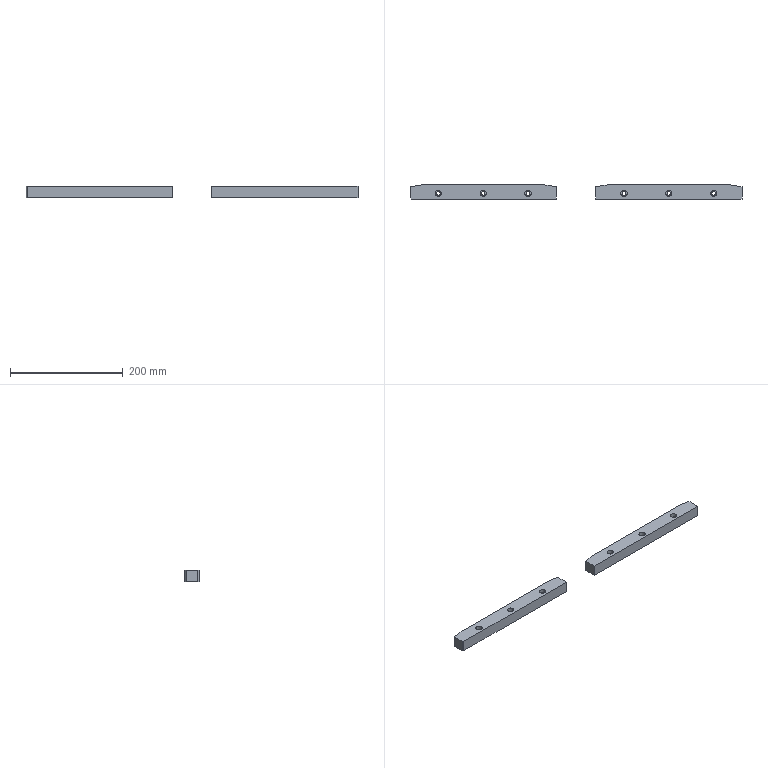Part | SolidWorks | features BaseBody 2 | 2 solids | 47 faces | box 588 x 25 x 20 mm | volume 249973 mm3 | cylinder 24 | plane 23 | commonest cylinder face diameters 6.6 x12 11 x12
STEP:
#1=CARTESIAN_POINT('',(180.,-11.723,13.2));
#2=VERTEX_POINT('',#1);
#3=CARTESIAN_POINT('',(191.,-11.723,13.2));
#4=VERTEX_POINT('',#3);
#5=CARTESIAN_POINT('',(185.5,-11.723,13.2));
#6=DIRECTION('',(0.,0.,1.));
#7=DIRECTION('',(1.,0.,0.));
#8=AXIS2_PLACEMENT_3D('',#5,#6,#7);
#9=CIRCLE('',#8,5.5);
#10=EDGE_CURVE('',#2,#4,#9,.T.);
#11=ORIENTED_EDGE('',*,*,#10,.F.);
#12=CARTESIAN_POINT('',(180.,-11.723,20.));
#13=VERTEX_POINT('',#12);
#14=CARTESIAN_POINT('',(180.,-11.723,20.));
#15=DIRECTION('',(0.,0.,1.));
#16=VECTOR('',#15,1000.);
#17=LINE('',#14,#16);
#18=EDGE_CURVE('',#2,#13,#17,.T.);
#19=ORIENTED_EDGE('',*,*,#18,.T.);
#20=CARTESIAN_POINT('',(191.,-11.723,20.));
#21=VERTEX_POINT('',#20);
#22=CARTESIAN_POINT('',(185.5,-11.723,20.));
#23=DIRECTION('',(0.,0.,1.));
#24=DIRECTION('',(1.,0.,0.));
#25=AXIS2_PLACEMENT_3D('',#22,#23,#24);
#26=CIRCLE('',#25,5.5);
#27=EDGE_CURVE('',#13,#21,#26,.T.);
#28=ORIENTED_EDGE('',*,*,#27,.T.);
#29=CARTESIAN_POINT('',(191.,-11.723,20.));
#30=DIRECTION('',(0.,0.,1.));
#31=VECTOR('',#30,1000.);
#32=LINE('',#29,#31);
#33=EDGE_CURVE('',#4,#21,#32,.T.);
#34=ORIENTED_EDGE('',*,*,#33,.F.);
#35=EDGE_LOOP('',(#11,#19,#28,#34));
#36=FACE_OUTER_BOUND('',#35,.T.);
#37=CARTESIAN_POINT('',(185.5,-11.723,20.));
#38=DIRECTION('',(0.,0.,1.));
#39=DIRECTION('',(1.,0.,0.));
#40=AXIS2_PLACEMENT_3D('',#37,#38,#39);
#41=CYLINDRICAL_SURFACE('',#40,5.5);
#42=ADVANCED_FACE('',(#36),#41,.F.);
#43=CARTESIAN_POINT('',(182.2,-11.723,0.));
#44=VERTEX_POINT('',#43);
#45=CARTESIAN_POINT('',(188.8,-11.723,0.));
#46=VERTEX_POINT('',#45);
#47=CARTESIAN_POINT('',(185.5,-11.723,0.));
#48=DIRECTION('',(0.,0.,1.));
#49=DIRECTION('',(1.,0.,0.));
#50=AXIS2_PLACEMENT_3D('',#47,#48,#49);
#51=CIRCLE('',#50,3.3);
#52=EDGE_CURVE('',#44,#46,#51,.T.);
#53=ORIENTED_EDGE('',*,*,#52,.F.);
#54=CARTESIAN_POINT('',(182.2,-11.723,13.2));
#55=VERTEX_POINT('',#54);
#56=CARTESIAN_POINT('',(182.2,-11.723,20.));
#57=DIRECTION('',(0.,0.,1.));
#58=VECTOR('',#57,1000.);
#59=LINE('',#56,#58);
#60=EDGE_CURVE('',#44,#55,#59,.T.);
#61=ORIENTED_EDGE('',*,*,#60,.T.);
#62=CARTESIAN_POINT('',(188.8,-11.723,13.2));
#63=VERTEX_POINT('',#62);
#64=CARTESIAN_POINT('',(185.5,-11.723,13.2));
#65=DIRECTION('',(0.,0.,1.));
#66=DIRECTION('',(1.,0.,0.));
#67=AXIS2_PLACEMENT_3D('',#64,#65,#66);
#68=CIRCLE('',#67,3.3);
#69=EDGE_CURVE('',#55,#63,#68,.T.);
#70=ORIENTED_EDGE('',*,*,#69,.T.);
#71=CARTESIAN_POINT('',(188.8,-11.723,20.));
#72=DIRECTION('',(0.,0.,1.));
#73=VECTOR('',#72,1000.);
#74=LINE('',#71,#73);
#75=EDGE_CURVE('',#46,#63,#74,.T.);
#76=ORIENTED_EDGE('',*,*,#75,.F.);
#77=EDGE_LOOP('',(#53,#61,#70,#76));
#78=FACE_OUTER_BOUND('',#77,.T.);
#79=CARTESIAN_POINT('',(185.5,-11.723,20.));
#80=DIRECTION('',(0.,0.,1.));
#81=DIRECTION('',(1.,0.,0.));
#82=AXIS2_PLACEMENT_3D('',#79,#80,#81);
#83=CYLINDRICAL_SURFACE('',#82,3.3);
#84=ADVANCED_FACE('',(#78),#83,.F.);
#85=CARTESIAN_POINT('',(259.5,-11.723,13.2));
#86=VERTEX_POINT('',#85);
#87=CARTESIAN_POINT('',(270.5,-11.723,13.2));
#88=VERTEX_POINT('',#87);
#89=CARTESIAN_POINT('',(265.,-11.723,13.2));
#90=DIRECTION('',(0.,0.,1.));
#91=DIRECTION('',(1.,0.,0.));
#92=AXIS2_PLACEMENT_3D('',#89,#90,#91);
#93=CIRCLE('',#92,5.5);
#94=EDGE_CURVE('',#86,#88,#93,.T.);
#95=ORIENTED_EDGE('',*,*,#94,.F.);
#96=CARTESIAN_POINT('',(259.5,-11.723,20.));
#97=VERTEX_POINT('',#96);
#98=CARTESIAN_POINT('',(259.5,-11.723,20.));
#99=DIRECTION('',(0.,0.,1.));
#100=VECTOR('',#99,1000.);
#101=LINE('',#98,#100);
#102=EDGE_CURVE('',#86,#97,#101,.T.);
#103=ORIENTED_EDGE('',*,*,#102,.T.);
#104=CARTESIAN_POINT('',(270.5,-11.723,20.));
#105=VERTEX_POINT('',#104);
#106=CARTESIAN_POINT('',(265.,-11.723,20.));
#107=DIRECTION('',(0.,0.,1.));
#108=DIRECTION('',(1.,0.,0.));
#109=AXIS2_PLACEMENT_3D('',#106,#107,#108);
#110=CIRCLE('',#109,5.5);
#111=EDGE_CURVE('',#97,#105,#110,.T.);
#112=ORIENTED_EDGE('',*,*,#111,.T.);
#113=CARTESIAN_POINT('',(270.5,-11.723,20.));
#114=DIRECTION('',(0.,0.,1.));
#115=VECTOR('',#114,1000.);
#116=LINE('',#113,#115);
#117=EDGE_CURVE('',#88,#105,#116,.T.);
#118=ORIENTED_EDGE('',*,*,#117,.F.);
#119=EDGE_LOOP('',(#95,#103,#112,#118));
#120=FACE_OUTER_BOUND('',#119,.T.);
#121=CARTESIAN_POINT('',(265.,-11.723,20.));
#122=DIRECTION('',(0.,0.,1.));
#123=DIRECTION('',(1.,0.,0.));
#124=AXIS2_PLACEMENT_3D('',#121,#122,#123);
#125=CYLINDRICAL_SURFACE('',#124,5.5);
#126=ADVANCED_FACE('',(#120),#125,.F.);
#127=CARTESIAN_POINT('',(261.7,-11.723,0.));
#128=VERTEX_POINT('',#127);
#129=CARTESIAN_POINT('',(268.3,-11.723,0.));
#130=VERTEX_POINT('',#129);
#131=CARTESIAN_POINT('',(265.,-11.723,0.));
#132=DIRECTION('',(0.,0.,1.));
#133=DIRECTION('',(1.,0.,0.));
#134=AXIS2_PLACEMENT_3D('',#131,#132,#133);
#135=CIRCLE('',#134,3.3);
#136=EDGE_CURVE('',#128,#130,#135,.T.);
#137=ORIENTED_EDGE('',*,*,#136,.F.);
#138=CARTESIAN_POINT('',(261.7,-11.723,13.2));
#139=VERTEX_POINT('',#138);
#140=CARTESIAN_POINT('',(261.7,-11.723,20.));
#141=DIRECTION('',(0.,0.,1.));
#142=VECTOR('',#141,1000.);
#143=LINE('',#140,#142);
#144=EDGE_CURVE('',#128,#139,#143,.T.);
#145=ORIENTED_EDGE('',*,*,#144,.T.);
#146=CARTESIAN_POINT('',(268.3,-11.723,13.2));
#147=VERTEX_POINT('',#146);
#148=CARTESIAN_POINT('',(265.,-11.723,13.2));
#149=DIRECTION('',(0.,0.,1.));
#150=DIRECTION('',(1.,0.,0.));
#151=AXIS2_PLACEMENT_3D('',#148,#149,#150);
#152=CIRCLE('',#151,3.3);
#153=EDGE_CURVE('',#139,#147,#152,.T.);
#154=ORIENTED_EDGE('',*,*,#153,.T.);
#155=CARTESIAN_POINT('',(268.3,-11.723,20.));
#156=DIRECTION('',(0.,0.,1.));
#157=VECTOR('',#156,1000.);
#158=LINE('',#155,#157);
#159=EDGE_CURVE('',#130,#147,#158,.T.);
#160=ORIENTED_EDGE('',*,*,#159,.F.);
#161=EDGE_LOOP('',(#137,#145,#154,#160));
#162=FACE_OUTER_BOUND('',#161,.T.);
#163=CARTESIAN_POINT('',(265.,-11.723,20.));
#164=DIRECTION('',(0.,0.,1.));
#165=DIRECTION('',(1.,0.,0.));
#166=AXIS2_PLACEMENT_3D('',#163,#164,#165);
#167=CYLINDRICAL_SURFACE('',#166,3.3);
#168=ADVANCED_FACE('',(#162),#167,.F.);
#169=CARTESIAN_POINT('',(100.5,-11.723,13.2));
#170=VERTEX_POINT('',#169);
#171=CARTESIAN_POINT('',(111.5,-11.723,13.2));
#172=VERTEX_POINT('',#171);
#173=CARTESIAN_POINT('',(106.,-11.723,13.2));
#174=DIRECTION('',(0.,0.,1.));
#175=DIRECTION('',(1.,0.,0.));
#176=AXIS2_PLACEMENT_3D('',#173,#174,#175);
#177=CIRCLE('',#176,5.5);
#178=EDGE_CURVE('',#170,#172,#177,.T.);
#179=ORIENTED_EDGE('',*,*,#178,.F.);
#180=CARTESIAN_POINT('',(100.5,-11.723,20.));
#181=VERTEX_POINT('',#180);
#182=CARTESIAN_POINT('',(100.5,-11.723,20.));
#183=DIRECTION('',(0.,0.,1.));
#184=VECTOR('',#183,1000.);
#185=LINE('',#182,#184);
#186=EDGE_CURVE('',#170,#181,#185,.T.);
#187=ORIENTED_EDGE('',*,*,#186,.T.);
#188=CARTESIAN_POINT('',(111.5,-11.723,20.));
#189=VERTEX_POINT('',#188);
#190=CARTESIAN_POINT('',(106.,-11.723,20.));
#191=DIRECTION('',(0.,0.,1.));
#192=DIRECTION('',(1.,0.,0.));
#193=AXIS2_PLACEMENT_3D('',#190,#191,#192);
#194=CIRCLE('',#193,5.5);
#195=EDGE_CURVE('',#181,#189,#194,.T.);
#196=ORIENTED_EDGE('',*,*,#195,.T.);
#197=CARTESIAN_POINT('',(111.5,-11.723,20.));
#198=DIRECTION('',(0.,0.,1.));
#199=VECTOR('',#198,1000.);
#200=LINE('',#197,#199);
#201=EDGE_CURVE('',#172,#189,#200,.T.);
#202=ORIENTED_EDGE('',*,*,#201,.F.);
#203=EDGE_LOOP('',(#179,#187,#196,#202));
#204=FACE_OUTER_BOUND('',#203,.T.);
#205=CARTESIAN_POINT('',(106.,-11.723,20.));
#206=DIRECTION('',(0.,0.,1.));
#207=DIRECTION('',(1.,0.,0.));
#208=AXIS2_PLACEMENT_3D('',#205,#206,#207);
#209=CYLINDRICAL_SURFACE('',#208,5.5);
#210=ADVANCED_FACE('',(#204),#209,.F.);
#211=CARTESIAN_POINT('',(102.7,-11.723,0.));
#212=VERTEX_POINT('',#211);
#213=CARTESIAN_POINT('',(109.3,-11.723,0.));
#214=VERTEX_POINT('',#213);
#215=CARTESIAN_POINT('',(106.,-11.723,0.));
#216=DIRECTION('',(0.,0.,1.));
#217=DIRECTION('',(1.,0.,0.));
#218=AXIS2_PLACEMENT_3D('',#215,#216,#217);
#219=CIRCLE('',#218,3.3);
#220=EDGE_CURVE('',#212,#214,#219,.T.);
#221=ORIENTED_EDGE('',*,*,#220,.F.);
#222=CARTESIAN_POINT('',(102.7,-11.723,13.2));
#223=VERTEX_POINT('',#222);
#224=CARTESIAN_POINT('',(102.7,-11.723,20.));
#225=DIRECTION('',(0.,0.,1.));
#226=VECTOR('',#225,1000.);
#227=LINE('',#224,#226);
#228=EDGE_CURVE('',#212,#223,#227,.T.);
#229=ORIENTED_EDGE('',*,*,#228,.T.);
#230=CARTESIAN_POINT('',(109.3,-11.723,13.2));
#231=VERTEX_POINT('',#230);
#232=CARTESIAN_POINT('',(106.,-11.723,13.2));
#233=DIRECTION('',(0.,0.,1.));
#234=DIRECTION('',(1.,0.,0.));
#235=AXIS2_PLACEMENT_3D('',#232,#233,#234);
#236=CIRCLE('',#235,3.3);
#237=EDGE_CURVE('',#223,#231,#236,.T.);
#238=ORIENTED_EDGE('',*,*,#237,.T.);
#239=CARTESIAN_POINT('',(109.3,-11.723,20.));
#240=DIRECTION('',(0.,0.,1.));
#241=VECTOR('',#240,1000.);
#242=LINE('',#239,#241);
#243=EDGE_CURVE('',#214,#231,#242,.T.);
#244=ORIENTED_EDGE('',*,*,#243,.F.);
#245=EDGE_LOOP('',(#221,#229,#238,#244));
#246=FACE_OUTER_BOUND('',#245,.T.);
#247=CARTESIAN_POINT('',(106.,-11.723,20.));
#248=DIRECTION('',(0.,0.,1.));
#249=DIRECTION('',(1.,0.,0.));
#250=AXIS2_PLACEMENT_3D('',#247,#248,#249);
#251=CYLINDRICAL_SURFACE('',#250,3.3);
#252=ADVANCED_FACE('',(#246),#251,.F.);
#253=CARTESIAN_POINT('',(295.,3.277,0.));
#254=VERTEX_POINT('',#253);
#255=CARTESIAN_POINT('',(76.,3.277,0.));
#256=VERTEX_POINT('',#255);
#257=CARTESIAN_POINT('',(-253.,3.277,0.));
#258=DIRECTION('',(-1.,0.,0.));
#259=VECTOR('',#258,1000.);
#260=LINE('',#257,#259);
#261=EDGE_CURVE('',#254,#256,#260,.T.);
#262=ORIENTED_EDGE('',*,*,#261,.T.);
#263=CARTESIAN_POINT('',(76.,3.277,20.));
#264=VERTEX_POINT('',#263);
#265=CARTESIAN_POINT('',(76.,3.277,20.));
#266=DIRECTION('',(0.,0.,1.));
#267=VECTOR('',#266,1000.);
#268=LINE('',#265,#267);
#269=EDGE_CURVE('',#256,#264,#268,.T.);
#270=ORIENTED_EDGE('',*,*,#269,.T.);
#271=CARTESIAN_POINT('',(295.,3.277,20.));
#272=VERTEX_POINT('',#271);
#273=CARTESIAN_POINT('',(-253.,3.277,20.));
#274=DIRECTION('',(-1.,0.,0.));
#275=VECTOR('',#274,1000.);
#276=LINE('',#273,#275);
#277=EDGE_CURVE('',#272,#264,#276,.T.);
#278=ORIENTED_EDGE('',*,*,#277,.F.);
#279=CARTESIAN_POINT('',(295.,3.277,20.));
#280=DIRECTION('',(0.,0.,-1.));
#281=VECTOR('',#280,1000.);
#282=LINE('',#279,#281);
#283=EDGE_CURVE('',#272,#254,#282,.T.);
#284=ORIENTED_EDGE('',*,*,#283,.T.);
#285=EDGE_LOOP('',(#262,#270,#278,#284));
#286=FACE_OUTER_BOUND('',#285,.T.);
#287=CARTESIAN_POINT('',(-253.,3.277,20.));
#288=DIRECTION('',(0.,-1.,0.));
#289=DIRECTION('',(1.,0.,0.));
#290=AXIS2_PLACEMENT_3D('',#287,#288,#289);
#291=PLANE('',#290);
#292=ADVANCED_FACE('',(#286),#291,.F.);
#293=CARTESIAN_POINT('',(56.,-21.723,20.));
#294=VERTEX_POINT('',#293);
#295=CARTESIAN_POINT('',(315.,-21.723,20.));
#296=VERTEX_POINT('',#295);
#297=CARTESIAN_POINT('',(-271.,-21.723,20.));
#298=DIRECTION('',(1.,0.,0.));
#299=VECTOR('',#298,1000.);
#300=LINE('',#297,#299);
#301=EDGE_CURVE('',#294,#296,#300,.T.);
#302=ORIENTED_EDGE('',*,*,#301,.F.);
#303=CARTESIAN_POINT('',(56.,-21.723,0.));
#304=VERTEX_POINT('',#303);
#305=CARTESIAN_POINT('',(56.,-21.723,20.));
#306=DIRECTION('',(0.,0.,-1.));
#307=VECTOR('',#306,1000.);
#308=LINE('',#305,#307);
#309=EDGE_CURVE('',#294,#304,#308,.T.);
#310=ORIENTED_EDGE('',*,*,#309,.T.);
#311=CARTESIAN_POINT('',(315.,-21.723,0.));
#312=VERTEX_POINT('',#311);
#313=CARTESIAN_POINT('',(-271.,-21.723,0.));
#314=DIRECTION('',(1.,0.,0.));
#315=VECTOR('',#314,1000.);
#316=LINE('',#313,#315);
#317=EDGE_CURVE('',#304,#312,#316,.T.);
#318=ORIENTED_EDGE('',*,*,#317,.T.);
#319=CARTESIAN_POINT('',(315.,-21.723,20.));
#320=DIRECTION('',(0.,0.,-1.));
#321=VECTOR('',#320,1000.);
#322=LINE('',#319,#321);
#323=EDGE_CURVE('',#296,#312,#322,.T.);
#324=ORIENTED_EDGE('',*,*,#323,.F.);
#325=EDGE_LOOP('',(#302,#310,#318,#324));
#326=FACE_OUTER_BOUND('',#325,.T.);
#327=CARTESIAN_POINT('',(-271.,-21.723,20.));
#328=DIRECTION('',(0.,1.,0.));
#329=DIRECTION('',(-1.,0.,0.));
#330=AXIS2_PLACEMENT_3D('',#327,#328,#329);
#331=PLANE('',#330);
#332=ADVANCED_FACE('',(#326),#331,.F.);
#333=CARTESIAN_POINT('',(106.,-11.723,20.));
#334=DIRECTION('',(0.,0.,1.));
#335=DIRECTION('',(1.,0.,0.));
#336=AXIS2_PLACEMENT_3D('',#333,#334,#335);
#337=CIRCLE('',#336,5.5);
#338=EDGE_CURVE('',#189,#181,#337,.T.);
#339=ORIENTED_EDGE('',*,*,#338,.F.);
#340=ORIENTED_EDGE('',*,*,#195,.F.);
#341=EDGE_LOOP('',(#339,#340));
#342=FACE_BOUND('',#341,.T.);
#343=CARTESIAN_POINT('',(265.,-11.723,20.));
#344=DIRECTION('',(0.,0.,1.));
#345=DIRECTION('',(1.,0.,0.));
#346=AXIS2_PLACEMENT_3D('',#343,#344,#345);
#347=CIRCLE('',#346,5.5);
#348=EDGE_CURVE('',#105,#97,#347,.T.);
#349=ORIENTED_EDGE('',*,*,#348,.F.);
#350=ORIENTED_EDGE('',*,*,#111,.F.);
#351=EDGE_LOOP('',(#349,#350));
#352=FACE_BOUND('',#351,.T.);
#353=CARTESIAN_POINT('',(185.5,-11.723,20.));
#354=DIRECTION('',(0.,0.,1.));
#355=DIRECTION('',(1.,0.,0.));
#356=AXIS2_PLACEMENT_3D('',#353,#354,#355);
#357=CIRCLE('',#356,5.5);
#358=EDGE_CURVE('',#21,#13,#357,.T.);
#359=ORIENTED_EDGE('',*,*,#358,.F.);
#360=ORIENTED_EDGE('',*,*,#27,.F.);
#361=EDGE_LOOP('',(#359,#360));
#362=FACE_BOUND('',#361,.T.);
#363=ORIENTED_EDGE('',*,*,#277,.T.);
#364=CARTESIAN_POINT('',(56.,0.2766,20.));
#365=VERTEX_POINT('',#364);
#366=CARTESIAN_POINT('',(76.,3.277,20.));
#367=DIRECTION('',(-0.9889,-0.1483,0.));
#368=VECTOR('',#367,1000.);
#369=LINE('',#366,#368);
#370=EDGE_CURVE('',#264,#365,#369,.T.);
#371=ORIENTED_EDGE('',*,*,#370,.T.);
#372=CARTESIAN_POINT('',(56.,-54.685,20.));
#373=DIRECTION('',(0.,1.,0.));
#374=VECTOR('',#373,1000.);
#375=LINE('',#372,#374);
#376=EDGE_CURVE('',#294,#365,#375,.T.);
#377=ORIENTED_EDGE('',*,*,#376,.F.);
#378=ORIENTED_EDGE('',*,*,#301,.T.);
#379=CARTESIAN_POINT('',(315.,0.2766,20.));
#380=VERTEX_POINT('',#379);
#381=CARTESIAN_POINT('',(315.,0.2766,20.));
#382=DIRECTION('',(0.,1.,0.));
#383=VECTOR('',#382,1000.);
#384=LINE('',#381,#383);
#385=EDGE_CURVE('',#296,#380,#384,.T.);
#386=ORIENTED_EDGE('',*,*,#385,.T.);
#387=CARTESIAN_POINT('',(295.,3.277,20.));
#388=DIRECTION('',(-0.9889,0.1483,0.));
#389=VECTOR('',#388,1000.);
#390=LINE('',#387,#389);
#391=EDGE_CURVE('',#380,#272,#390,.T.);
#392=ORIENTED_EDGE('',*,*,#391,.T.);
#393=EDGE_LOOP('',(#363,#371,#377,#378,#386,#392));
#394=FACE_OUTER_BOUND('',#393,.T.);
#395=CARTESIAN_POINT('',(0.,0.,20.));
#396=DIRECTION('',(0.,0.,-1.));
#397=DIRECTION('',(-1.,0.,0.));
#398=AXIS2_PLACEMENT_3D('',#395,#396,#397);
#399=PLANE('',#398);
#400=ADVANCED_FACE('',(#342,#352,#362,#394),#399,.F.);
#401=CARTESIAN_POINT('',(56.,0.2766,0.));
#402=VERTEX_POINT('',#401);
#403=CARTESIAN_POINT('',(56.,0.,0.));
#404=DIRECTION('',(0.,-1.,0.));
#405=VECTOR('',#404,1000.);
#406=LINE('',#403,#405);
#407=EDGE_CURVE('',#402,#304,#406,.T.);
#408=ORIENTED_EDGE('',*,*,#407,.F.);
#409=CARTESIAN_POINT('',(1.192,-7.945,0.));
#410=DIRECTION('',(0.9889,0.1483,0.));
#411=VECTOR('',#410,1000.);
#412=LINE('',#409,#411);
#413=EDGE_CURVE('',#402,#256,#412,.T.);
#414=ORIENTED_EDGE('',*,*,#413,.T.);
#415=ORIENTED_EDGE('',*,*,#261,.F.);
#416=CARTESIAN_POINT('',(315.,0.2766,0.));
#417=VERTEX_POINT('',#416);
#418=CARTESIAN_POINT('',(295.,3.277,0.));
#419=DIRECTION('',(-0.9889,0.1483,0.));
#420=VECTOR('',#419,1000.);
#421=LINE('',#418,#420);
#422=EDGE_CURVE('',#417,#254,#421,.T.);
#423=ORIENTED_EDGE('',*,*,#422,.F.);
#424=CARTESIAN_POINT('',(315.,0.2766,0.));
#425=DIRECTION('',(0.,1.,0.));
#426=VECTOR('',#425,1000.);
#427=LINE('',#424,#426);
#428=EDGE_CURVE('',#312,#417,#427,.T.);
#429=ORIENTED_EDGE('',*,*,#428,.F.);
#430=ORIENTED_EDGE('',*,*,#317,.F.);
#431=EDGE_LOOP('',(#408,#414,#415,#423,#429,#430));
#432=FACE_OUTER_BOUND('',#431,.T.);
#433=CARTESIAN_POINT('',(106.,-11.723,0.));
#434=DIRECTION('',(0.,0.,1.));
#435=DIRECTION('',(1.,0.,0.));
#436=AXIS2_PLACEMENT_3D('',#433,#434,#435);
#437=CIRCLE('',#436,3.3);
#438=EDGE_CURVE('',#214,#212,#437,.T.);
#439=ORIENTED_EDGE('',*,*,#438,.T.);
#440=ORIENTED_EDGE('',*,*,#220,.T.);
#441=EDGE_LOOP('',(#439,#440));
#442=FACE_BOUND('',#441,.T.);
#443=CARTESIAN_POINT('',(265.,-11.723,0.));
#444=DIRECTION('',(0.,0.,1.));
#445=DIRECTION('',(1.,0.,0.));
#446=AXIS2_PLACEMENT_3D('',#443,#444,#445);
#447=CIRCLE('',#446,3.3);
#448=EDGE_CURVE('',#130,#128,#447,.T.);
#449=ORIENTED_EDGE('',*,*,#448,.T.);
#450=ORIENTED_EDGE('',*,*,#136,.T.);
#451=EDGE_LOOP('',(#449,#450));
#452=FACE_BOUND('',#451,.T.);
#453=CARTESIAN_POINT('',(185.5,-11.723,0.));
#454=DIRECTION('',(0.,0.,1.));
#455=DIRECTION('',(1.,0.,0.));
#456=AXIS2_PLACEMENT_3D('',#453,#454,#455);
#457=CIRCLE('',#456,3.3);
#458=EDGE_CURVE('',#46,#44,#457,.T.);
#459=ORIENTED_EDGE('',*,*,#458,.T.);
#460=ORIENTED_EDGE('',*,*,#52,.T.);
#461=EDGE_LOOP('',(#459,#460));
#462=FACE_BOUND('',#461,.T.);
#463=CARTESIAN_POINT('',(0.,0.,0.));
#464=DIRECTION('',(0.,0.,-1.));
#465=DIRECTION('',(-1.,0.,0.));
#466=AXIS2_PLACEMENT_3D('',#463,#464,#465);
#467=PLANE('',#466);
#468=ADVANCED_FACE('',(#432,#442,#452,#462),#467,.T.);
#469=ORIENTED_EDGE('',*,*,#422,.T.);
#470=ORIENTED_EDGE('',*,*,#283,.F.);
#471=ORIENTED_EDGE('',*,*,#391,.F.);
#472=CARTESIAN_POINT('',(315.,0.2766,20.));
#473=DIRECTION('',(0.,0.,-1.));
#474=VECTOR('',#473,1000.);
#475=LINE('',#472,#474);
#476=EDGE_CURVE('',#380,#417,#475,.T.);
#477=ORIENTED_EDGE('',*,*,#476,.T.);
#478=EDGE_LOOP('',(#469,#470,#471,#477));
#479=FACE_OUTER_BOUND('',#478,.T.);
#480=CARTESIAN_POINT('',(295.,3.277,20.));
#481=DIRECTION('',(-0.1483,-0.9889,0.));
#482=DIRECTION('',(0.9889,-0.1483,0.));
#483=AXIS2_PLACEMENT_3D('',#480,#481,#482);
#484=PLANE('',#483);
#485=ADVANCED_FACE('',(#479),#484,.F.);
#486=ORIENTED_EDGE('',*,*,#428,.T.);
#487=ORIENTED_EDGE('',*,*,#476,.F.);
#488=ORIENTED_EDGE('',*,*,#385,.F.);
#489=ORIENTED_EDGE('',*,*,#323,.T.);
#490=EDGE_LOOP('',(#486,#487,#488,#489));
#491=FACE_OUTER_BOUND('',#490,.T.);
#492=CARTESIAN_POINT('',(315.,0.2766,20.));
#493=DIRECTION('',(-1.,0.,0.));
#494=DIRECTION('',(0.,-1.,0.));
#495=AXIS2_PLACEMENT_3D('',#492,#493,#494);
#496=PLANE('',#495);
#497=ADVANCED_FACE('',(#491),#496,.F.);
#498=ORIENTED_EDGE('',*,*,#228,.F.);
#499=ORIENTED_EDGE('',*,*,#438,.F.);
#500=ORIENTED_EDGE('',*,*,#243,.T.);
#501=CARTESIAN_POINT('',(106.,-11.723,13.2));
#502=DIRECTION('',(0.,0.,1.));
#503=DIRECTION('',(1.,0.,0.));
#504=AXIS2_PLACEMENT_3D('',#501,#502,#503);
#505=CIRCLE('',#504,3.3);
#506=EDGE_CURVE('',#231,#223,#505,.T.);
#507=ORIENTED_EDGE('',*,*,#506,.T.);
#508=EDGE_LOOP('',(#498,#499,#500,#507));
#509=FACE_OUTER_BOUND('',#508,.T.);
#510=CARTESIAN_POINT('',(106.,-11.723,20.));
#511=DIRECTION('',(0.,0.,1.));
#512=DIRECTION('',(1.,0.,0.));
#513=AXIS2_PLACEMENT_3D('',#510,#511,#512);
#514=CYLINDRICAL_SURFACE('',#513,3.3);
#515=ADVANCED_FACE('',(#509),#514,.F.);
#516=ORIENTED_EDGE('',*,*,#506,.F.);
#517=ORIENTED_EDGE('',*,*,#237,.F.);
#518=EDGE_LOOP('',(#516,#517));
#519=FACE_BOUND('',#518,.T.);
#520=CARTESIAN_POINT('',(106.,-11.723,13.2));
#521=DIRECTION('',(0.,0.,1.));
#522=DIRECTION('',(1.,0.,0.));
#523=AXIS2_PLACEMENT_3D('',#520,#521,#522);
#524=CIRCLE('',#523,5.5);
#525=EDGE_CURVE('',#172,#170,#524,.T.);
#526=ORIENTED_EDGE('',*,*,#525,.T.);
#527=ORIENTED_EDGE('',*,*,#178,.T.);
#528=EDGE_LOOP('',(#526,#527));
#529=FACE_OUTER_BOUND('',#528,.T.);
#530=CARTESIAN_POINT('',(109.3,-11.723,13.2));
#531=DIRECTION('',(0.,0.,-1.));
#532=DIRECTION('',(-1.,0.,0.));
#533=AXIS2_PLACEMENT_3D('',#530,#531,#532);
#534=PLANE('',#533);
#535=ADVANCED_FACE('',(#519,#529),#534,.F.);
#536=ORIENTED_EDGE('',*,*,#186,.F.);
#537=ORIENTED_EDGE('',*,*,#525,.F.);
#538=ORIENTED_EDGE('',*,*,#201,.T.);
#539=ORIENTED_EDGE('',*,*,#338,.T.);
#540=EDGE_LOOP('',(#536,#537,#538,#539));
#541=FACE_OUTER_BOUND('',#540,.T.);
#542=CARTESIAN_POINT('',(106.,-11.723,20.));
#543=DIRECTION('',(0.,0.,1.));
#544=DIRECTION('',(1.,0.,0.));
#545=AXIS2_PLACEMENT_3D('',#542,#543,#544);
#546=CYLINDRICAL_SURFACE('',#545,5.5);
#547=ADVANCED_FACE('',(#541),#546,.F.);
#548=ORIENTED_EDGE('',*,*,#144,.F.);
#549=ORIENTED_EDGE('',*,*,#448,.F.);
#550=ORIENTED_EDGE('',*,*,#159,.T.);
#551=CARTESIAN_POINT('',(265.,-11.723,13.2));
#552=DIRECTION('',(0.,0.,1.));
#553=DIRECTION('',(1.,0.,0.));
#554=AXIS2_PLACEMENT_3D('',#551,#552,#553);
#555=CIRCLE('',#554,3.3);
#556=EDGE_CURVE('',#147,#139,#555,.T.);
#557=ORIENTED_EDGE('',*,*,#556,.T.);
#558=EDGE_LOOP('',(#548,#549,#550,#557));
#559=FACE_OUTER_BOUND('',#558,.T.);
#560=CARTESIAN_POINT('',(265.,-11.723,20.));
#561=DIRECTION('',(0.,0.,1.));
#562=DIRECTION('',(1.,0.,0.));
#563=AXIS2_PLACEMENT_3D('',#560,#561,#562);
#564=CYLINDRICAL_SURFACE('',#563,3.3);
#565=ADVANCED_FACE('',(#559),#564,.F.);
#566=ORIENTED_EDGE('',*,*,#556,.F.);
#567=ORIENTED_EDGE('',*,*,#153,.F.);
#568=EDGE_LOOP('',(#566,#567));
#569=FACE_BOUND('',#568,.T.);
#570=CARTESIAN_POINT('',(265.,-11.723,13.2));
#571=DIRECTION('',(0.,0.,1.));
#572=DIRECTION('',(1.,0.,0.));
#573=AXIS2_PLACEMENT_3D('',#570,#571,#572);
#574=CIRCLE('',#573,5.5);
#575=EDGE_CURVE('',#88,#86,#574,.T.);
#576=ORIENTED_EDGE('',*,*,#575,.T.);
#577=ORIENTED_EDGE('',*,*,#94,.T.);
#578=EDGE_LOOP('',(#576,#577));
#579=FACE_OUTER_BOUND('',#578,.T.);
#580=CARTESIAN_POINT('',(268.3,-11.723,13.2));
#581=DIRECTION('',(0.,0.,-1.));
#582=DIRECTION('',(-1.,0.,0.));
#583=AXIS2_PLACEMENT_3D('',#580,#581,#582);
#584=PLANE('',#583);
#585=ADVANCED_FACE('',(#569,#579),#584,.F.);
#586=ORIENTED_EDGE('',*,*,#102,.F.);
#587=ORIENTED_EDGE('',*,*,#575,.F.);
#588=ORIENTED_EDGE('',*,*,#117,.T.);
#589=ORIENTED_EDGE('',*,*,#348,.T.);
#590=EDGE_LOOP('',(#586,#587,#588,#589));
#591=FACE_OUTER_BOUND('',#590,.T.);
#592=CARTESIAN_POINT('',(265.,-11.723,20.));
#593=DIRECTION('',(0.,0.,1.));
#594=DIRECTION('',(1.,0.,0.));
#595=AXIS2_PLACEMENT_3D('',#592,#593,#594);
#596=CYLINDRICAL_SURFACE('',#595,5.5);
#597=ADVANCED_FACE('',(#591),#596,.F.);
#598=ORIENTED_EDGE('',*,*,#60,.F.);
#599=ORIENTED_EDGE('',*,*,#458,.F.);
#600=ORIENTED_EDGE('',*,*,#75,.T.);
#601=CARTESIAN_POINT('',(185.5,-11.723,13.2));
#602=DIRECTION('',(0.,0.,1.));
#603=DIRECTION('',(1.,0.,0.));
#604=AXIS2_PLACEMENT_3D('',#601,#602,#603);
#605=CIRCLE('',#604,3.3);
#606=EDGE_CURVE('',#63,#55,#605,.T.);
#607=ORIENTED_EDGE('',*,*,#606,.T.);
#608=EDGE_LOOP('',(#598,#599,#600,#607));
#609=FACE_OUTER_BOUND('',#608,.T.);
#610=CARTESIAN_POINT('',(185.5,-11.723,20.));
#611=DIRECTION('',(0.,0.,1.));
#612=DIRECTION('',(1.,0.,0.));
#613=AXIS2_PLACEMENT_3D('',#610,#611,#612);
#614=CYLINDRICAL_SURFACE('',#613,3.3);
#615=ADVANCED_FACE('',(#609),#614,.F.);
#616=ORIENTED_EDGE('',*,*,#606,.F.);
#617=ORIENTED_EDGE('',*,*,#69,.F.);
#618=EDGE_LOOP('',(#616,#617));
#619=FACE_BOUND('',#618,.T.);
#620=CARTESIAN_POINT('',(185.5,-11.723,13.2));
#621=DIRECTION('',(0.,0.,1.));
#622=DIRECTION('',(1.,0.,0.));
#623=AXIS2_PLACEMENT_3D('',#620,#621,#622);
#624=CIRCLE('',#623,5.5);
#625=EDGE_CURVE('',#4,#2,#624,.T.);
#626=ORIENTED_EDGE('',*,*,#625,.T.);
#627=ORIENTED_EDGE('',*,*,#10,.T.);
#628=EDGE_LOOP('',(#626,#627));
#629=FACE_OUTER_BOUND('',#628,.T.);
#630=CARTESIAN_POINT('',(188.8,-11.723,13.2));
#631=DIRECTION('',(0.,0.,-1.));
#632=DIRECTION('',(-1.,0.,0.));
#633=AXIS2_PLACEMENT_3D('',#630,#631,#632);
#634=PLANE('',#633);
#635=ADVANCED_FACE('',(#619,#629),#634,.F.);
#636=ORIENTED_EDGE('',*,*,#18,.F.);
#637=ORIENTED_EDGE('',*,*,#625,.F.);
#638=ORIENTED_EDGE('',*,*,#33,.T.);
#639=ORIENTED_EDGE('',*,*,#358,.T.);
#640=EDGE_LOOP('',(#636,#637,#638,#639));
#641=FACE_OUTER_BOUND('',#640,.T.);
#642=CARTESIAN_POINT('',(185.5,-11.723,20.));
#643=DIRECTION('',(0.,0.,1.));
#644=DIRECTION('',(1.,0.,0.));
#645=AXIS2_PLACEMENT_3D('',#642,#643,#644);
#646=CYLINDRICAL_SURFACE('',#645,5.5);
#647=ADVANCED_FACE('',(#641),#646,.F.);
#648=ORIENTED_EDGE('',*,*,#376,.T.);
#649=CARTESIAN_POINT('',(56.,0.2766,0.));
#650=DIRECTION('',(0.,0.,-1.));
#651=VECTOR('',#650,1000.);
#652=LINE('',#649,#651);
#653=EDGE_CURVE('',#365,#402,#652,.T.);
#654=ORIENTED_EDGE('',*,*,#653,.T.);
#655=ORIENTED_EDGE('',*,*,#407,.T.);
#656=ORIENTED_EDGE('',*,*,#309,.F.);
#657=EDGE_LOOP('',(#648,#654,#655,#656));
#658=FACE_OUTER_BOUND('',#657,.T.);
#659=CARTESIAN_POINT('',(56.,-54.685,0.));
#660=DIRECTION('',(1.,0.,0.));
#661=DIRECTION('',(0.,0.,-1.));
#662=AXIS2_PLACEMENT_3D('',#659,#660,#661);
#663=PLANE('',#662);
#664=ADVANCED_FACE('',(#658),#663,.F.);
#665=ORIENTED_EDGE('',*,*,#413,.F.);
#666=ORIENTED_EDGE('',*,*,#653,.F.);
#667=ORIENTED_EDGE('',*,*,#370,.F.);
#668=ORIENTED_EDGE('',*,*,#269,.F.);
#669=EDGE_LOOP('',(#665,#666,#667,#668));
#670=FACE_OUTER_BOUND('',#669,.T.);
#671=CARTESIAN_POINT('',(76.,3.277,20.));
#672=DIRECTION('',(0.1483,-0.9889,0.));
#673=DIRECTION('',(0.,0.,1.));
#674=AXIS2_PLACEMENT_3D('',#671,#672,#673);
#675=PLANE('',#674);
#676=ADVANCED_FACE('',(#670),#675,.F.);
#677=CLOSED_SHELL('',(#42,#84,#126,#168,#210,#252,#292,#332,#400,#468,#485,#497,#515,#535,#547,#565,#585,#597,#615,#635,#647,#664,#676));
#678=MANIFOLD_SOLID_BREP('',#677);
#679=CARTESIAN_POINT('',(-226.3,-11.723,0.));
#680=VERTEX_POINT('',#679);
#681=CARTESIAN_POINT('',(-219.7,-11.723,0.));
#682=VERTEX_POINT('',#681);
#683=CARTESIAN_POINT('',(-223.,-11.723,0.));
#684=DIRECTION('',(0.,0.,1.));
#685=DIRECTION('',(1.,0.,0.));
#686=AXIS2_PLACEMENT_3D('',#683,#684,#685);
#687=CIRCLE('',#686,3.3);
#688=EDGE_CURVE('',#680,#682,#687,.T.);
#689=ORIENTED_EDGE('',*,*,#688,.F.);
#690=CARTESIAN_POINT('',(-226.3,-11.723,13.2));
#691=VERTEX_POINT('',#690);
#692=CARTESIAN_POINT('',(-226.3,-11.723,20.));
#693=DIRECTION('',(0.,0.,1.));
#694=VECTOR('',#693,1000.);
#695=LINE('',#692,#694);
#696=EDGE_CURVE('',#680,#691,#695,.T.);
#697=ORIENTED_EDGE('',*,*,#696,.T.);
#698=CARTESIAN_POINT('',(-219.7,-11.723,13.2));
#699=VERTEX_POINT('',#698);
#700=CARTESIAN_POINT('',(-223.,-11.723,13.2));
#701=DIRECTION('',(0.,0.,1.));
#702=DIRECTION('',(1.,0.,0.));
#703=AXIS2_PLACEMENT_3D('',#700,#701,#702);
#704=CIRCLE('',#703,3.3);
#705=EDGE_CURVE('',#691,#699,#704,.T.);
#706=ORIENTED_EDGE('',*,*,#705,.T.);
#707=CARTESIAN_POINT('',(-219.7,-11.723,20.));
#708=DIRECTION('',(0.,0.,1.));
#709=VECTOR('',#708,1000.);
#710=LINE('',#707,#709);
#711=EDGE_CURVE('',#682,#699,#710,.T.);
#712=ORIENTED_EDGE('',*,*,#711,.F.);
#713=EDGE_LOOP('',(#689,#697,#706,#712));
#714=FACE_OUTER_BOUND('',#713,.T.);
#715=CARTESIAN_POINT('',(-223.,-11.723,20.));
#716=DIRECTION('',(0.,0.,1.));
#717=DIRECTION('',(1.,0.,0.));
#718=AXIS2_PLACEMENT_3D('',#715,#716,#717);
#719=CYLINDRICAL_SURFACE('',#718,3.3);
#720=ADVANCED_FACE('',(#714),#719,.F.);
#721=CARTESIAN_POINT('',(-146.8,-11.723,0.));
#722=VERTEX_POINT('',#721);
#723=CARTESIAN_POINT('',(-140.2,-11.723,0.));
#724=VERTEX_POINT('',#723);
#725=CARTESIAN_POINT('',(-143.5,-11.723,0.));
#726=DIRECTION('',(0.,0.,1.));
#727=DIRECTION('',(1.,0.,0.));
#728=AXIS2_PLACEMENT_3D('',#725,#726,#727);
#729=CIRCLE('',#728,3.3);
#730=EDGE_CURVE('',#722,#724,#729,.T.);
#731=ORIENTED_EDGE('',*,*,#730,.F.);
#732=CARTESIAN_POINT('',(-146.8,-11.723,13.2));
#733=VERTEX_POINT('',#732);
#734=CARTESIAN_POINT('',(-146.8,-11.723,20.));
#735=DIRECTION('',(0.,0.,1.));
#736=VECTOR('',#735,1000.);
#737=LINE('',#734,#736);
#738=EDGE_CURVE('',#722,#733,#737,.T.);
#739=ORIENTED_EDGE('',*,*,#738,.T.);
#740=CARTESIAN_POINT('',(-140.2,-11.723,13.2));
#741=VERTEX_POINT('',#740);
#742=CARTESIAN_POINT('',(-143.5,-11.723,13.2));
#743=DIRECTION('',(0.,0.,1.));
#744=DIRECTION('',(1.,0.,0.));
#745=AXIS2_PLACEMENT_3D('',#742,#743,#744);
#746=CIRCLE('',#745,3.3);
#747=EDGE_CURVE('',#733,#741,#746,.T.);
#748=ORIENTED_EDGE('',*,*,#747,.T.);
#749=CARTESIAN_POINT('',(-140.2,-11.723,20.));
#750=DIRECTION('',(0.,0.,1.));
#751=VECTOR('',#750,1000.);
#752=LINE('',#749,#751);
#753=EDGE_CURVE('',#724,#741,#752,.T.);
#754=ORIENTED_EDGE('',*,*,#753,.F.);
#755=EDGE_LOOP('',(#731,#739,#748,#754));
#756=FACE_OUTER_BOUND('',#755,.T.);
#757=CARTESIAN_POINT('',(-143.5,-11.723,20.));
#758=DIRECTION('',(0.,0.,1.));
#759=DIRECTION('',(1.,0.,0.));
#760=AXIS2_PLACEMENT_3D('',#757,#758,#759);
#761=CYLINDRICAL_SURFACE('',#760,3.3);
#762=ADVANCED_FACE('',(#756),#761,.F.);
#763=CARTESIAN_POINT('',(-67.3,-11.723,0.));
#764=VERTEX_POINT('',#763);
#765=CARTESIAN_POINT('',(-60.7,-11.723,0.));
#766=VERTEX_POINT('',#765);
#767=CARTESIAN_POINT('',(-64.,-11.723,0.));
#768=DIRECTION('',(0.,0.,1.));
#769=DIRECTION('',(1.,0.,0.));
#770=AXIS2_PLACEMENT_3D('',#767,#768,#769);
#771=CIRCLE('',#770,3.3);
#772=EDGE_CURVE('',#764,#766,#771,.T.);
#773=ORIENTED_EDGE('',*,*,#772,.F.);
#774=CARTESIAN_POINT('',(-67.3,-11.723,13.2));
#775=VERTEX_POINT('',#774);
#776=CARTESIAN_POINT('',(-67.3,-11.723,20.));
#777=DIRECTION('',(0.,0.,1.));
#778=VECTOR('',#777,1000.);
#779=LINE('',#776,#778);
#780=EDGE_CURVE('',#764,#775,#779,.T.);
#781=ORIENTED_EDGE('',*,*,#780,.T.);
#782=CARTESIAN_POINT('',(-60.7,-11.723,13.2));
#783=VERTEX_POINT('',#782);
#784=CARTESIAN_POINT('',(-64.,-11.723,13.2));
#785=DIRECTION('',(0.,0.,1.));
#786=DIRECTION('',(1.,0.,0.));
#787=AXIS2_PLACEMENT_3D('',#784,#785,#786);
#788=CIRCLE('',#787,3.3);
#789=EDGE_CURVE('',#775,#783,#788,.T.);
#790=ORIENTED_EDGE('',*,*,#789,.T.);
#791=CARTESIAN_POINT('',(-60.7,-11.723,20.));
#792=DIRECTION('',(0.,0.,1.));
#793=VECTOR('',#792,1000.);
#794=LINE('',#791,#793);
#795=EDGE_CURVE('',#766,#783,#794,.T.);
#796=ORIENTED_EDGE('',*,*,#795,.F.);
#797=EDGE_LOOP('',(#773,#781,#790,#796));
#798=FACE_OUTER_BOUND('',#797,.T.);
#799=CARTESIAN_POINT('',(-64.,-11.723,20.));
#800=DIRECTION('',(0.,0.,1.));
#801=DIRECTION('',(1.,0.,0.));
#802=AXIS2_PLACEMENT_3D('',#799,#800,#801);
#803=CYLINDRICAL_SURFACE('',#802,3.3);
#804=ADVANCED_FACE('',(#798),#803,.F.);
#805=CARTESIAN_POINT('',(-228.5,-11.723,13.2));
#806=VERTEX_POINT('',#805);
#807=CARTESIAN_POINT('',(-217.5,-11.723,13.2));
#808=VERTEX_POINT('',#807);
#809=CARTESIAN_POINT('',(-223.,-11.723,13.2));
#810=DIRECTION('',(0.,0.,1.));
#811=DIRECTION('',(1.,0.,0.));
#812=AXIS2_PLACEMENT_3D('',#809,#810,#811);
#813=CIRCLE('',#812,5.5);
#814=EDGE_CURVE('',#806,#808,#813,.T.);
#815=ORIENTED_EDGE('',*,*,#814,.F.);
#816=CARTESIAN_POINT('',(-228.5,-11.723,20.));
#817=VERTEX_POINT('',#816);
#818=CARTESIAN_POINT('',(-228.5,-11.723,20.));
#819=DIRECTION('',(0.,0.,1.));
#820=VECTOR('',#819,1000.);
#821=LINE('',#818,#820);
#822=EDGE_CURVE('',#806,#817,#821,.T.);
#823=ORIENTED_EDGE('',*,*,#822,.T.);
#824=CARTESIAN_POINT('',(-217.5,-11.723,20.));
#825=VERTEX_POINT('',#824);
#826=CARTESIAN_POINT('',(-223.,-11.723,20.));
#827=DIRECTION('',(0.,0.,1.));
#828=DIRECTION('',(1.,0.,0.));
#829=AXIS2_PLACEMENT_3D('',#826,#827,#828);
#830=CIRCLE('',#829,5.5);
#831=EDGE_CURVE('',#817,#825,#830,.T.);
#832=ORIENTED_EDGE('',*,*,#831,.T.);
#833=CARTESIAN_POINT('',(-217.5,-11.723,20.));
#834=DIRECTION('',(0.,0.,1.));
#835=VECTOR('',#834,1000.);
#836=LINE('',#833,#835);
#837=EDGE_CURVE('',#808,#825,#836,.T.);
#838=ORIENTED_EDGE('',*,*,#837,.F.);
#839=EDGE_LOOP('',(#815,#823,#832,#838));
#840=FACE_OUTER_BOUND('',#839,.T.);
#841=CARTESIAN_POINT('',(-223.,-11.723,20.));
#842=DIRECTION('',(0.,0.,1.));
#843=DIRECTION('',(1.,0.,0.));
#844=AXIS2_PLACEMENT_3D('',#841,#842,#843);
#845=CYLINDRICAL_SURFACE('',#844,5.5);
#846=ADVANCED_FACE('',(#840),#845,.F.);
#847=CARTESIAN_POINT('',(-149.,-11.723,13.2));
#848=VERTEX_POINT('',#847);
#849=CARTESIAN_POINT('',(-138.,-11.723,13.2));
#850=VERTEX_POINT('',#849);
#851=CARTESIAN_POINT('',(-143.5,-11.723,13.2));
#852=DIRECTION('',(0.,0.,1.));
#853=DIRECTION('',(1.,0.,0.));
#854=AXIS2_PLACEMENT_3D('',#851,#852,#853);
#855=CIRCLE('',#854,5.5);
#856=EDGE_CURVE('',#848,#850,#855,.T.);
#857=ORIENTED_EDGE('',*,*,#856,.F.);
#858=CARTESIAN_POINT('',(-149.,-11.723,20.));
#859=VERTEX_POINT('',#858);
#860=CARTESIAN_POINT('',(-149.,-11.723,20.));
#861=DIRECTION('',(0.,0.,1.));
#862=VECTOR('',#861,1000.);
#863=LINE('',#860,#862);
#864=EDGE_CURVE('',#848,#859,#863,.T.);
#865=ORIENTED_EDGE('',*,*,#864,.T.);
#866=CARTESIAN_POINT('',(-138.,-11.723,20.));
#867=VERTEX_POINT('',#866);
#868=CARTESIAN_POINT('',(-143.5,-11.723,20.));
#869=DIRECTION('',(0.,0.,1.));
#870=DIRECTION('',(1.,0.,0.));
#871=AXIS2_PLACEMENT_3D('',#868,#869,#870);
#872=CIRCLE('',#871,5.5);
#873=EDGE_CURVE('',#859,#867,#872,.T.);
#874=ORIENTED_EDGE('',*,*,#873,.T.);
#875=CARTESIAN_POINT('',(-138.,-11.723,20.));
#876=DIRECTION('',(0.,0.,1.));
#877=VECTOR('',#876,1000.);
#878=LINE('',#875,#877);
#879=EDGE_CURVE('',#850,#867,#878,.T.);
#880=ORIENTED_EDGE('',*,*,#879,.F.);
#881=EDGE_LOOP('',(#857,#865,#874,#880));
#882=FACE_OUTER_BOUND('',#881,.T.);
#883=CARTESIAN_POINT('',(-143.5,-11.723,20.));
#884=DIRECTION('',(0.,0.,1.));
#885=DIRECTION('',(1.,0.,0.));
#886=AXIS2_PLACEMENT_3D('',#883,#884,#885);
#887=CYLINDRICAL_SURFACE('',#886,5.5);
#888=ADVANCED_FACE('',(#882),#887,.F.);
#889=CARTESIAN_POINT('',(-69.5,-11.723,13.2));
#890=VERTEX_POINT('',#889);
#891=CARTESIAN_POINT('',(-58.5,-11.723,13.2));
#892=VERTEX_POINT('',#891);
#893=CARTESIAN_POINT('',(-64.,-11.723,13.2));
#894=DIRECTION('',(0.,0.,1.));
#895=DIRECTION('',(1.,0.,0.));
#896=AXIS2_PLACEMENT_3D('',#893,#894,#895);
#897=CIRCLE('',#896,5.5);
#898=EDGE_CURVE('',#890,#892,#897,.T.);
#899=ORIENTED_EDGE('',*,*,#898,.F.);
#900=CARTESIAN_POINT('',(-69.5,-11.723,20.));
#901=VERTEX_POINT('',#900);
#902=CARTESIAN_POINT('',(-69.5,-11.723,20.));
#903=DIRECTION('',(0.,0.,1.));
#904=VECTOR('',#903,1000.);
#905=LINE('',#902,#904);
#906=EDGE_CURVE('',#890,#901,#905,.T.);
#907=ORIENTED_EDGE('',*,*,#906,.T.);
#908=CARTESIAN_POINT('',(-58.5,-11.723,20.));
#909=VERTEX_POINT('',#908);
#910=CARTESIAN_POINT('',(-64.,-11.723,20.));
#911=DIRECTION('',(0.,0.,1.));
#912=DIRECTION('',(1.,0.,0.));
#913=AXIS2_PLACEMENT_3D('',#910,#911,#912);
#914=CIRCLE('',#913,5.5);
#915=EDGE_CURVE('',#901,#909,#914,.T.);
#916=ORIENTED_EDGE('',*,*,#915,.T.);
#917=CARTESIAN_POINT('',(-58.5,-11.723,20.));
#918=DIRECTION('',(0.,0.,1.));
#919=VECTOR('',#918,1000.);
#920=LINE('',#917,#919);
#921=EDGE_CURVE('',#892,#909,#920,.T.);
#922=ORIENTED_EDGE('',*,*,#921,.F.);
#923=EDGE_LOOP('',(#899,#907,#916,#922));
#924=FACE_OUTER_BOUND('',#923,.T.);
#925=CARTESIAN_POINT('',(-64.,-11.723,20.));
#926=DIRECTION('',(0.,0.,1.));
#927=DIRECTION('',(1.,0.,0.));
#928=AXIS2_PLACEMENT_3D('',#925,#926,#927);
#929=CYLINDRICAL_SURFACE('',#928,5.5);
#930=ADVANCED_FACE('',(#924),#929,.F.);
#931=CARTESIAN_POINT('',(-64.,-11.723,13.2));
#932=DIRECTION('',(0.,0.,1.));
#933=DIRECTION('',(1.,0.,0.));
#934=AXIS2_PLACEMENT_3D('',#931,#932,#933);
#935=CIRCLE('',#934,3.3);
#936=EDGE_CURVE('',#783,#775,#935,.T.);
#937=ORIENTED_EDGE('',*,*,#936,.F.);
#938=ORIENTED_EDGE('',*,*,#789,.F.);
#939=EDGE_LOOP('',(#937,#938));
#940=FACE_BOUND('',#939,.T.);
#941=CARTESIAN_POINT('',(-64.,-11.723,13.2));
#942=DIRECTION('',(0.,0.,1.));
#943=DIRECTION('',(1.,0.,0.));
#944=AXIS2_PLACEMENT_3D('',#941,#942,#943);
#945=CIRCLE('',#944,5.5);
#946=EDGE_CURVE('',#892,#890,#945,.T.);
#947=ORIENTED_EDGE('',*,*,#946,.T.);
#948=ORIENTED_EDGE('',*,*,#898,.T.);
#949=EDGE_LOOP('',(#947,#948));
#950=FACE_OUTER_BOUND('',#949,.T.);
#951=CARTESIAN_POINT('',(-60.7,-11.723,13.2));
#952=DIRECTION('',(0.,0.,-1.));
#953=DIRECTION('',(-1.,0.,0.));
#954=AXIS2_PLACEMENT_3D('',#951,#952,#953);
#955=PLANE('',#954);
#956=ADVANCED_FACE('',(#940,#950),#955,.F.);
#957=CARTESIAN_POINT('',(-143.5,-11.723,13.2));
#958=DIRECTION('',(0.,0.,1.));
#959=DIRECTION('',(1.,0.,0.));
#960=AXIS2_PLACEMENT_3D('',#957,#958,#959);
#961=CIRCLE('',#960,3.3);
#962=EDGE_CURVE('',#741,#733,#961,.T.);
#963=ORIENTED_EDGE('',*,*,#962,.F.);
#964=ORIENTED_EDGE('',*,*,#747,.F.);
#965=EDGE_LOOP('',(#963,#964));
#966=FACE_BOUND('',#965,.T.);
#967=CARTESIAN_POINT('',(-143.5,-11.723,13.2));
#968=DIRECTION('',(0.,0.,1.));
#969=DIRECTION('',(1.,0.,0.));
#970=AXIS2_PLACEMENT_3D('',#967,#968,#969);
#971=CIRCLE('',#970,5.5);
#972=EDGE_CURVE('',#850,#848,#971,.T.);
#973=ORIENTED_EDGE('',*,*,#972,.T.);
#974=ORIENTED_EDGE('',*,*,#856,.T.);
#975=EDGE_LOOP('',(#973,#974));
#976=FACE_OUTER_BOUND('',#975,.T.);
#977=CARTESIAN_POINT('',(-140.2,-11.723,13.2));
#978=DIRECTION('',(0.,0.,-1.));
#979=DIRECTION('',(-1.,0.,0.));
#980=AXIS2_PLACEMENT_3D('',#977,#978,#979);
#981=PLANE('',#980);
#982=ADVANCED_FACE('',(#966,#976),#981,.F.);
#983=CARTESIAN_POINT('',(-223.,-11.723,13.2));
#984=DIRECTION('',(0.,0.,1.));
#985=DIRECTION('',(1.,0.,0.));
#986=AXIS2_PLACEMENT_3D('',#983,#984,#985);
#987=CIRCLE('',#986,3.3);
#988=EDGE_CURVE('',#699,#691,#987,.T.);
#989=ORIENTED_EDGE('',*,*,#988,.F.);
#990=ORIENTED_EDGE('',*,*,#705,.F.);
#991=EDGE_LOOP('',(#989,#990));
#992=FACE_BOUND('',#991,.T.);
#993=CARTESIAN_POINT('',(-223.,-11.723,13.2));
#994=DIRECTION('',(0.,0.,1.));
#995=DIRECTION('',(1.,0.,0.));
#996=AXIS2_PLACEMENT_3D('',#993,#994,#995);
#997=CIRCLE('',#996,5.5);
#998=EDGE_CURVE('',#808,#806,#997,.T.);
#999=ORIENTED_EDGE('',*,*,#998,.T.);
#1000=ORIENTED_EDGE('',*,*,#814,.T.);
#1001=EDGE_LOOP('',(#999,#1000));
#1002=FACE_OUTER_BOUND('',#1001,.T.);
#1003=CARTESIAN_POINT('',(-219.7,-11.723,13.2));
#1004=DIRECTION('',(0.,0.,-1.));
#1005=DIRECTION('',(-1.,0.,0.));
#1006=AXIS2_PLACEMENT_3D('',#1003,#1004,#1005);
#1007=PLANE('',#1006);
#1008=ADVANCED_FACE('',(#992,#1002),#1007,.F.);
#1009=ORIENTED_EDGE('',*,*,#906,.F.);
#1010=ORIENTED_EDGE('',*,*,#946,.F.);
#1011=ORIENTED_EDGE('',*,*,#921,.T.);
#1012=CARTESIAN_POINT('',(-64.,-11.723,20.));
#1013=DIRECTION('',(0.,0.,1.));
#1014=DIRECTION('',(1.,0.,0.));
#1015=AXIS2_PLACEMENT_3D('',#1012,#1013,#1014);
#1016=CIRCLE('',#1015,5.5);
#1017=EDGE_CURVE('',#909,#901,#1016,.T.);
#1018=ORIENTED_EDGE('',*,*,#1017,.T.);
#1019=EDGE_LOOP('',(#1009,#1010,#1011,#1018));
#1020=FACE_OUTER_BOUND('',#1019,.T.);
#1021=CARTESIAN_POINT('',(-64.,-11.723,20.));
#1022=DIRECTION('',(0.,0.,1.));
#1023=DIRECTION('',(1.,0.,0.));
#1024=AXIS2_PLACEMENT_3D('',#1021,#1022,#1023);
#1025=CYLINDRICAL_SURFACE('',#1024,5.5);
#1026=ADVANCED_FACE('',(#1020),#1025,.F.);
#1027=ORIENTED_EDGE('',*,*,#864,.F.);
#1028=ORIENTED_EDGE('',*,*,#972,.F.);
#1029=ORIENTED_EDGE('',*,*,#879,.T.);
#1030=CARTESIAN_POINT('',(-143.5,-11.723,20.));
#1031=DIRECTION('',(0.,0.,1.));
#1032=DIRECTION('',(1.,0.,0.));
#1033=AXIS2_PLACEMENT_3D('',#1030,#1031,#1032);
#1034=CIRCLE('',#1033,5.5);
#1035=EDGE_CURVE('',#867,#859,#1034,.T.);
#1036=ORIENTED_EDGE('',*,*,#1035,.T.);
#1037=EDGE_LOOP('',(#1027,#1028,#1029,#1036));
#1038=FACE_OUTER_BOUND('',#1037,.T.);
#1039=CARTESIAN_POINT('',(-143.5,-11.723,20.));
#1040=DIRECTION('',(0.,0.,1.));
#1041=DIRECTION('',(1.,0.,0.));
#1042=AXIS2_PLACEMENT_3D('',#1039,#1040,#1041);
#1043=CYLINDRICAL_SURFACE('',#1042,5.5);
#1044=ADVANCED_FACE('',(#1038),#1043,.F.);
#1045=ORIENTED_EDGE('',*,*,#822,.F.);
#1046=ORIENTED_EDGE('',*,*,#998,.F.);
#1047=ORIENTED_EDGE('',*,*,#837,.T.);
#1048=CARTESIAN_POINT('',(-223.,-11.723,20.));
#1049=DIRECTION('',(0.,0.,1.));
#1050=DIRECTION('',(1.,0.,0.));
#1051=AXIS2_PLACEMENT_3D('',#1048,#1049,#1050);
#1052=CIRCLE('',#1051,5.5);
#1053=EDGE_CURVE('',#825,#817,#1052,.T.);
#1054=ORIENTED_EDGE('',*,*,#1053,.T.);
#1055=EDGE_LOOP('',(#1045,#1046,#1047,#1054));
#1056=FACE_OUTER_BOUND('',#1055,.T.);
#1057=CARTESIAN_POINT('',(-223.,-11.723,20.));
#1058=DIRECTION('',(0.,0.,1.));
#1059=DIRECTION('',(1.,0.,0.));
#1060=AXIS2_PLACEMENT_3D('',#1057,#1058,#1059);
#1061=CYLINDRICAL_SURFACE('',#1060,5.5);
#1062=ADVANCED_FACE('',(#1056),#1061,.F.);
#1063=ORIENTED_EDGE('',*,*,#780,.F.);
#1064=CARTESIAN_POINT('',(-64.,-11.723,0.));
#1065=DIRECTION('',(0.,0.,1.));
#1066=DIRECTION('',(1.,0.,0.));
#1067=AXIS2_PLACEMENT_3D('',#1064,#1065,#1066);
#1068=CIRCLE('',#1067,3.3);
#1069=EDGE_CURVE('',#766,#764,#1068,.T.);
#1070=ORIENTED_EDGE('',*,*,#1069,.F.);
#1071=ORIENTED_EDGE('',*,*,#795,.T.);
#1072=ORIENTED_EDGE('',*,*,#936,.T.);
#1073=EDGE_LOOP('',(#1063,#1070,#1071,#1072));
#1074=FACE_OUTER_BOUND('',#1073,.T.);
#1075=CARTESIAN_POINT('',(-64.,-11.723,20.));
#1076=DIRECTION('',(0.,0.,1.));
#1077=DIRECTION('',(1.,0.,0.));
#1078=AXIS2_PLACEMENT_3D('',#1075,#1076,#1077);
#1079=CYLINDRICAL_SURFACE('',#1078,3.3);
#1080=ADVANCED_FACE('',(#1074),#1079,.F.);
#1081=ORIENTED_EDGE('',*,*,#738,.F.);
#1082=CARTESIAN_POINT('',(-143.5,-11.723,0.));
#1083=DIRECTION('',(0.,0.,1.));
#1084=DIRECTION('',(1.,0.,0.));
#1085=AXIS2_PLACEMENT_3D('',#1082,#1083,#1084);
#1086=CIRCLE('',#1085,3.3);
#1087=EDGE_CURVE('',#724,#722,#1086,.T.);
#1088=ORIENTED_EDGE('',*,*,#1087,.F.);
#1089=ORIENTED_EDGE('',*,*,#753,.T.);
#1090=ORIENTED_EDGE('',*,*,#962,.T.);
#1091=EDGE_LOOP('',(#1081,#1088,#1089,#1090));
#1092=FACE_OUTER_BOUND('',#1091,.T.);
#1093=CARTESIAN_POINT('',(-143.5,-11.723,20.));
#1094=DIRECTION('',(0.,0.,1.));
#1095=DIRECTION('',(1.,0.,0.));
#1096=AXIS2_PLACEMENT_3D('',#1093,#1094,#1095);
#1097=CYLINDRICAL_SURFACE('',#1096,3.3);
#1098=ADVANCED_FACE('',(#1092),#1097,.F.);
#1099=ORIENTED_EDGE('',*,*,#696,.F.);
#1100=CARTESIAN_POINT('',(-223.,-11.723,0.));
#1101=DIRECTION('',(0.,0.,1.));
#1102=DIRECTION('',(1.,0.,0.));
#1103=AXIS2_PLACEMENT_3D('',#1100,#1101,#1102);
#1104=CIRCLE('',#1103,3.3);
#1105=EDGE_CURVE('',#682,#680,#1104,.T.);
#1106=ORIENTED_EDGE('',*,*,#1105,.F.);
#1107=ORIENTED_EDGE('',*,*,#711,.T.);
#1108=ORIENTED_EDGE('',*,*,#988,.T.);
#1109=EDGE_LOOP('',(#1099,#1106,#1107,#1108));
#1110=FACE_OUTER_BOUND('',#1109,.T.);
#1111=CARTESIAN_POINT('',(-223.,-11.723,20.));
#1112=DIRECTION('',(0.,0.,1.));
#1113=DIRECTION('',(1.,0.,0.));
#1114=AXIS2_PLACEMENT_3D('',#1111,#1112,#1113);
#1115=CYLINDRICAL_SURFACE('',#1114,3.3);
#1116=ADVANCED_FACE('',(#1110),#1115,.F.);
#1117=CARTESIAN_POINT('',(-253.,3.277,0.));
#1118=VERTEX_POINT('',#1117);
#1119=CARTESIAN_POINT('',(-273.,0.2766,0.));
#1120=VERTEX_POINT('',#1119);
#1121=CARTESIAN_POINT('',(-273.,0.2766,0.));
#1122=DIRECTION('',(-0.9889,-0.1483,0.));
#1123=VECTOR('',#1122,1000.);
#1124=LINE('',#1121,#1123);
#1125=EDGE_CURVE('',#1118,#1120,#1124,.T.);
#1126=ORIENTED_EDGE('',*,*,#1125,.T.);
#1127=CARTESIAN_POINT('',(-273.,0.2766,20.));
#1128=VERTEX_POINT('',#1127);
#1129=CARTESIAN_POINT('',(-273.,0.2766,20.));
#1130=DIRECTION('',(0.,0.,-1.));
#1131=VECTOR('',#1130,1000.);
#1132=LINE('',#1129,#1131);
#1133=EDGE_CURVE('',#1128,#1120,#1132,.T.);
#1134=ORIENTED_EDGE('',*,*,#1133,.F.);
#1135=CARTESIAN_POINT('',(-253.,3.277,20.));
#1136=VERTEX_POINT('',#1135);
#1137=CARTESIAN_POINT('',(-273.,0.2766,20.));
#1138=DIRECTION('',(-0.9889,-0.1483,0.));
#1139=VECTOR('',#1138,1000.);
#1140=LINE('',#1137,#1139);
#1141=EDGE_CURVE('',#1136,#1128,#1140,.T.);
#1142=ORIENTED_EDGE('',*,*,#1141,.F.);
#1143=CARTESIAN_POINT('',(-253.,3.277,20.));
#1144=DIRECTION('',(0.,0.,-1.));
#1145=VECTOR('',#1144,1000.);
#1146=LINE('',#1143,#1145);
#1147=EDGE_CURVE('',#1136,#1118,#1146,.T.);
#1148=ORIENTED_EDGE('',*,*,#1147,.T.);
#1149=EDGE_LOOP('',(#1126,#1134,#1142,#1148));
#1150=FACE_OUTER_BOUND('',#1149,.T.);
#1151=CARTESIAN_POINT('',(-273.,0.2766,20.));
#1152=DIRECTION('',(0.1483,-0.9889,0.));
#1153=DIRECTION('',(0.9889,0.1483,0.));
#1154=AXIS2_PLACEMENT_3D('',#1151,#1152,#1153);
#1155=PLANE('',#1154);
#1156=ADVANCED_FACE('',(#1150),#1155,.F.);
#1157=CARTESIAN_POINT('',(-273.,-19.723,0.));
#1158=VERTEX_POINT('',#1157);
#1159=CARTESIAN_POINT('',(-273.,0.2766,0.));
#1160=DIRECTION('',(0.,-1.,0.));
#1161=VECTOR('',#1160,1000.);
#1162=LINE('',#1159,#1161);
#1163=EDGE_CURVE('',#1120,#1158,#1162,.T.);
#1164=ORIENTED_EDGE('',*,*,#1163,.T.);
#1165=CARTESIAN_POINT('',(-273.,-19.723,20.));
#1166=VERTEX_POINT('',#1165);
#1167=CARTESIAN_POINT('',(-273.,-19.723,20.));
#1168=DIRECTION('',(0.,0.,-1.));
#1169=VECTOR('',#1168,1000.);
#1170=LINE('',#1167,#1169);
#1171=EDGE_CURVE('',#1166,#1158,#1170,.T.);
#1172=ORIENTED_EDGE('',*,*,#1171,.F.);
#1173=CARTESIAN_POINT('',(-273.,0.2766,20.));
#1174=DIRECTION('',(0.,-1.,0.));
#1175=VECTOR('',#1174,1000.);
#1176=LINE('',#1173,#1175);
#1177=EDGE_CURVE('',#1128,#1166,#1176,.T.);
#1178=ORIENTED_EDGE('',*,*,#1177,.F.);
#1179=ORIENTED_EDGE('',*,*,#1133,.T.);
#1180=EDGE_LOOP('',(#1164,#1172,#1178,#1179));
#1181=FACE_OUTER_BOUND('',#1180,.T.);
#1182=CARTESIAN_POINT('',(-273.,0.2766,20.));
#1183=DIRECTION('',(1.,0.,0.));
#1184=DIRECTION('',(0.,0.,-1.));
#1185=AXIS2_PLACEMENT_3D('',#1182,#1183,#1184);
#1186=PLANE('',#1185);
#1187=ADVANCED_FACE('',(#1181),#1186,.F.);
#1188=CARTESIAN_POINT('',(-271.,-21.723,0.));
#1189=VERTEX_POINT('',#1188);
#1190=CARTESIAN_POINT('',(-273.,-19.723,0.));
#1191=DIRECTION('',(0.7071,-0.7071,0.));
#1192=VECTOR('',#1191,1000.);
#1193=LINE('',#1190,#1192);
#1194=EDGE_CURVE('',#1158,#1189,#1193,.T.);
#1195=ORIENTED_EDGE('',*,*,#1194,.T.);
#1196=CARTESIAN_POINT('',(-271.,-21.723,20.));
#1197=VERTEX_POINT('',#1196);
#1198=CARTESIAN_POINT('',(-271.,-21.723,20.));
#1199=DIRECTION('',(0.,0.,-1.));
#1200=VECTOR('',#1199,1000.);
#1201=LINE('',#1198,#1200);
#1202=EDGE_CURVE('',#1197,#1189,#1201,.T.);
#1203=ORIENTED_EDGE('',*,*,#1202,.F.);
#1204=CARTESIAN_POINT('',(-273.,-19.723,20.));
#1205=DIRECTION('',(0.7071,-0.7071,0.));
#1206=VECTOR('',#1205,1000.);
#1207=LINE('',#1204,#1206);
#1208=EDGE_CURVE('',#1166,#1197,#1207,.T.);
#1209=ORIENTED_EDGE('',*,*,#1208,.F.);
#1210=ORIENTED_EDGE('',*,*,#1171,.T.);
#1211=EDGE_LOOP('',(#1195,#1203,#1209,#1210));
#1212=FACE_OUTER_BOUND('',#1211,.T.);
#1213=CARTESIAN_POINT('',(-273.,-19.723,20.));
#1214=DIRECTION('',(0.7071,0.7071,0.));
#1215=DIRECTION('',(-0.7071,0.7071,0.));
#1216=AXIS2_PLACEMENT_3D('',#1213,#1214,#1215);
#1217=PLANE('',#1216);
#1218=ADVANCED_FACE('',(#1212),#1217,.F.);
#1219=ORIENTED_EDGE('',*,*,#1053,.F.);
#1220=ORIENTED_EDGE('',*,*,#831,.F.);
#1221=EDGE_LOOP('',(#1219,#1220));
#1222=FACE_BOUND('',#1221,.T.);
#1223=ORIENTED_EDGE('',*,*,#1035,.F.);
#1224=ORIENTED_EDGE('',*,*,#873,.F.);
#1225=EDGE_LOOP('',(#1223,#1224));
#1226=FACE_BOUND('',#1225,.T.);
#1227=ORIENTED_EDGE('',*,*,#1017,.F.);
#1228=ORIENTED_EDGE('',*,*,#915,.F.);
#1229=EDGE_LOOP('',(#1227,#1228));
#1230=FACE_BOUND('',#1229,.T.);
#1231=CARTESIAN_POINT('',(-14.,0.2766,20.));
#1232=VERTEX_POINT('',#1231);
#1233=CARTESIAN_POINT('',(-14.,-21.723,20.));
#1234=VERTEX_POINT('',#1233);
#1235=CARTESIAN_POINT('',(-14.,-54.685,20.));
#1236=DIRECTION('',(0.,-1.,0.));
#1237=VECTOR('',#1236,1000.);
#1238=LINE('',#1235,#1237);
#1239=EDGE_CURVE('',#1232,#1234,#1238,.T.);
#1240=ORIENTED_EDGE('',*,*,#1239,.F.);
#1241=CARTESIAN_POINT('',(-34.,3.277,20.));
#1242=VERTEX_POINT('',#1241);
#1243=CARTESIAN_POINT('',(-34.,3.277,20.));
#1244=DIRECTION('',(-0.9889,0.1483,0.));
#1245=VECTOR('',#1244,1000.);
#1246=LINE('',#1243,#1245);
#1247=EDGE_CURVE('',#1232,#1242,#1246,.T.);
#1248=ORIENTED_EDGE('',*,*,#1247,.T.);
#1249=CARTESIAN_POINT('',(-253.,3.277,20.));
#1250=DIRECTION('',(-1.,0.,0.));
#1251=VECTOR('',#1250,1000.);
#1252=LINE('',#1249,#1251);
#1253=EDGE_CURVE('',#1242,#1136,#1252,.T.);
#1254=ORIENTED_EDGE('',*,*,#1253,.T.);
#1255=ORIENTED_EDGE('',*,*,#1141,.T.);
#1256=ORIENTED_EDGE('',*,*,#1177,.T.);
#1257=ORIENTED_EDGE('',*,*,#1208,.T.);
#1258=CARTESIAN_POINT('',(-271.,-21.723,20.));
#1259=DIRECTION('',(1.,0.,0.));
#1260=VECTOR('',#1259,1000.);
#1261=LINE('',#1258,#1260);
#1262=EDGE_CURVE('',#1197,#1234,#1261,.T.);
#1263=ORIENTED_EDGE('',*,*,#1262,.T.);
#1264=EDGE_LOOP('',(#1240,#1248,#1254,#1255,#1256,#1257,#1263));
#1265=FACE_OUTER_BOUND('',#1264,.T.);
#1266=CARTESIAN_POINT('',(0.,0.,20.));
#1267=DIRECTION('',(0.,0.,-1.));
#1268=DIRECTION('',(-1.,0.,0.));
#1269=AXIS2_PLACEMENT_3D('',#1266,#1267,#1268);
#1270=PLANE('',#1269);
#1271=ADVANCED_FACE('',(#1222,#1226,#1230,#1265),#1270,.F.);
#1272=CARTESIAN_POINT('',(-34.,3.277,0.));
#1273=VERTEX_POINT('',#1272);
#1274=CARTESIAN_POINT('',(-253.,3.277,0.));
#1275=DIRECTION('',(-1.,0.,0.));
#1276=VECTOR('',#1275,1000.);
#1277=LINE('',#1274,#1276);
#1278=EDGE_CURVE('',#1273,#1118,#1277,.T.);
#1279=ORIENTED_EDGE('',*,*,#1278,.F.);
#1280=CARTESIAN_POINT('',(-14.,0.2766,0.));
#1281=VERTEX_POINT('',#1280);
#1282=CARTESIAN_POINT('',(-0.2675,-1.783,0.));
#1283=DIRECTION('',(0.9889,-0.1483,0.));
#1284=VECTOR('',#1283,1000.);
#1285=LINE('',#1282,#1284);
#1286=EDGE_CURVE('',#1273,#1281,#1285,.T.);
#1287=ORIENTED_EDGE('',*,*,#1286,.T.);
#1288=CARTESIAN_POINT('',(-14.,-21.723,0.));
#1289=VERTEX_POINT('',#1288);
#1290=CARTESIAN_POINT('',(-14.,0.,0.));
#1291=DIRECTION('',(0.,1.,0.));
#1292=VECTOR('',#1291,1000.);
#1293=LINE('',#1290,#1292);
#1294=EDGE_CURVE('',#1289,#1281,#1293,.T.);
#1295=ORIENTED_EDGE('',*,*,#1294,.F.);
#1296=CARTESIAN_POINT('',(-271.,-21.723,0.));
#1297=DIRECTION('',(1.,0.,0.));
#1298=VECTOR('',#1297,1000.);
#1299=LINE('',#1296,#1298);
#1300=EDGE_CURVE('',#1189,#1289,#1299,.T.);
#1301=ORIENTED_EDGE('',*,*,#1300,.F.);
#1302=ORIENTED_EDGE('',*,*,#1194,.F.);
#1303=ORIENTED_EDGE('',*,*,#1163,.F.);
#1304=ORIENTED_EDGE('',*,*,#1125,.F.);
#1305=EDGE_LOOP('',(#1279,#1287,#1295,#1301,#1302,#1303,#1304));
#1306=FACE_OUTER_BOUND('',#1305,.T.);
#1307=ORIENTED_EDGE('',*,*,#1105,.T.);
#1308=ORIENTED_EDGE('',*,*,#688,.T.);
#1309=EDGE_LOOP('',(#1307,#1308));
#1310=FACE_BOUND('',#1309,.T.);
#1311=ORIENTED_EDGE('',*,*,#1087,.T.);
#1312=ORIENTED_EDGE('',*,*,#730,.T.);
#1313=EDGE_LOOP('',(#1311,#1312));
#1314=FACE_BOUND('',#1313,.T.);
#1315=ORIENTED_EDGE('',*,*,#1069,.T.);
#1316=ORIENTED_EDGE('',*,*,#772,.T.);
#1317=EDGE_LOOP('',(#1315,#1316));
#1318=FACE_BOUND('',#1317,.T.);
#1319=CARTESIAN_POINT('',(0.,0.,0.));
#1320=DIRECTION('',(0.,0.,-1.));
#1321=DIRECTION('',(-1.,0.,0.));
#1322=AXIS2_PLACEMENT_3D('',#1319,#1320,#1321);
#1323=PLANE('',#1322);
#1324=ADVANCED_FACE('',(#1306,#1310,#1314,#1318),#1323,.T.);
#1325=ORIENTED_EDGE('',*,*,#1300,.T.);
#1326=CARTESIAN_POINT('',(-14.,-21.723,20.));
#1327=DIRECTION('',(0.,0.,1.));
#1328=VECTOR('',#1327,1000.);
#1329=LINE('',#1326,#1328);
#1330=EDGE_CURVE('',#1289,#1234,#1329,.T.);
#1331=ORIENTED_EDGE('',*,*,#1330,.T.);
#1332=ORIENTED_EDGE('',*,*,#1262,.F.);
#1333=ORIENTED_EDGE('',*,*,#1202,.T.);
#1334=EDGE_LOOP('',(#1325,#1331,#1332,#1333));
#1335=FACE_OUTER_BOUND('',#1334,.T.);
#1336=CARTESIAN_POINT('',(-271.,-21.723,20.));
#1337=DIRECTION('',(0.,1.,0.));
#1338=DIRECTION('',(-1.,0.,0.));
#1339=AXIS2_PLACEMENT_3D('',#1336,#1337,#1338);
#1340=PLANE('',#1339);
#1341=ADVANCED_FACE('',(#1335),#1340,.F.);
#1342=ORIENTED_EDGE('',*,*,#1253,.F.);
#1343=CARTESIAN_POINT('',(-34.,3.277,20.));
#1344=DIRECTION('',(0.,0.,-1.));
#1345=VECTOR('',#1344,1000.);
#1346=LINE('',#1343,#1345);
#1347=EDGE_CURVE('',#1242,#1273,#1346,.T.);
#1348=ORIENTED_EDGE('',*,*,#1347,.T.);
#1349=ORIENTED_EDGE('',*,*,#1278,.T.);
#1350=ORIENTED_EDGE('',*,*,#1147,.F.);
#1351=EDGE_LOOP('',(#1342,#1348,#1349,#1350));
#1352=FACE_OUTER_BOUND('',#1351,.T.);
#1353=CARTESIAN_POINT('',(-253.,3.277,20.));
#1354=DIRECTION('',(0.,-1.,0.));
#1355=DIRECTION('',(1.,0.,0.));
#1356=AXIS2_PLACEMENT_3D('',#1353,#1354,#1355);
#1357=PLANE('',#1356);
#1358=ADVANCED_FACE('',(#1352),#1357,.F.);
#1359=ORIENTED_EDGE('',*,*,#1294,.T.);
#1360=CARTESIAN_POINT('',(-14.,0.2766,0.));
#1361=DIRECTION('',(0.,0.,1.));
#1362=VECTOR('',#1361,1000.);
#1363=LINE('',#1360,#1362);
#1364=EDGE_CURVE('',#1281,#1232,#1363,.T.);
#1365=ORIENTED_EDGE('',*,*,#1364,.T.);
#1366=ORIENTED_EDGE('',*,*,#1239,.T.);
#1367=ORIENTED_EDGE('',*,*,#1330,.F.);
#1368=EDGE_LOOP('',(#1359,#1365,#1366,#1367));
#1369=FACE_OUTER_BOUND('',#1368,.T.);
#1370=CARTESIAN_POINT('',(-14.,-54.685,0.));
#1371=DIRECTION('',(-1.,0.,0.));
#1372=DIRECTION('',(0.,0.,1.));
#1373=AXIS2_PLACEMENT_3D('',#1370,#1371,#1372);
#1374=PLANE('',#1373);
#1375=ADVANCED_FACE('',(#1369),#1374,.F.);
#1376=ORIENTED_EDGE('',*,*,#1247,.F.);
#1377=ORIENTED_EDGE('',*,*,#1364,.F.);
#1378=ORIENTED_EDGE('',*,*,#1286,.F.);
#1379=ORIENTED_EDGE('',*,*,#1347,.F.);
#1380=EDGE_LOOP('',(#1376,#1377,#1378,#1379));
#1381=FACE_OUTER_BOUND('',#1380,.T.);
#1382=CARTESIAN_POINT('',(-34.,3.277,20.));
#1383=DIRECTION('',(-0.1483,-0.9889,0.));
#1384=DIRECTION('',(0.,0.,-1.));
#1385=AXIS2_PLACEMENT_3D('',#1382,#1383,#1384);
#1386=PLANE('',#1385);
#1387=ADVANCED_FACE('',(#1381),#1386,.F.);
#1388=CLOSED_SHELL('',(#720,#762,#804,#846,#888,#930,#956,#982,#1008,#1026,#1044,#1062,#1080,#1098,#1116,#1156,#1187,#1218,#1271,#1324,#1341,#1358,#1375,#1387));
#1389=MANIFOLD_SOLID_BREP('',#1388);
#1390=CARTESIAN_POINT('',(0.,0.,0.));
#1391=DIRECTION('',(0.,0.,1.));
#1392=DIRECTION('',(1.,0.,0.));
#1393=AXIS2_PLACEMENT_3D('',#1390,#1391,#1392);
#1394=(LENGTH_UNIT()NAMED_UNIT(*)SI_UNIT(.MILLI.,.METRE.));
#1395=UNCERTAINTY_MEASURE_WITH_UNIT(LENGTH_MEASURE(0.00001),#1394,'','');
#1396=(NAMED_UNIT(*)PLANE_ANGLE_UNIT()SI_UNIT($,.RADIAN.));
#1397=(NAMED_UNIT(*)SI_UNIT($,.STERADIAN.)SOLID_ANGLE_UNIT());
#1398=(GEOMETRIC_REPRESENTATION_CONTEXT(3)GLOBAL_UNCERTAINTY_ASSIGNED_CONTEXT((#1395))GLOBAL_UNIT_ASSIGNED_CONTEXT((#1394,#1396,#1397))REPRESENTATION_CONTEXT('',''));
#1399=ADVANCED_BREP_SHAPE_REPRESENTATION('',(#678,#1389,#1393),#1398);